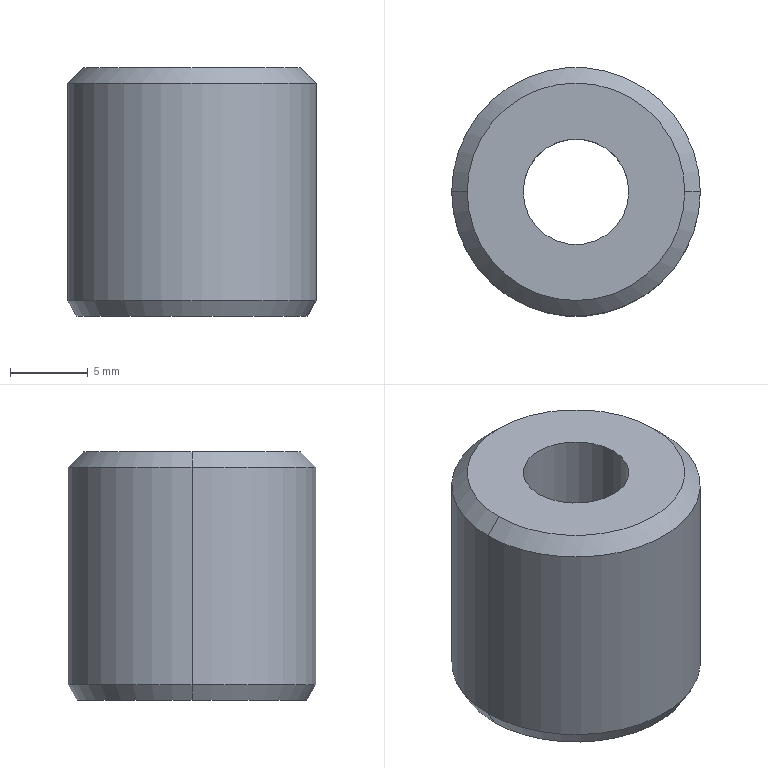Part | NX | features DCBA16_1 2 | 1 solid | 13 faces | box 16 x 16 x 16 mm | volume 2062 mm3 | cone 6 | cylinder 4 | plane 3 | commonest cylinder face diameters 16 x2 6.806 x1 11 x1
STEP:
#1=CARTESIAN_POINT('',(1522.268,-24.022,-21.001));
#2=VERTEX_POINT('',#1);
#3=CARTESIAN_POINT('',(1521.69,-24.022,-20.001));
#4=VERTEX_POINT('',#3);
#5=CARTESIAN_POINT('',(1521.69,-24.022,-20.001));
#6=DIRECTION('',(-0.5,0.,0.866));
#7=VECTOR('',#6,1000.);
#8=LINE('',#5,#7);
#9=EDGE_CURVE('',#2,#4,#8,.T.);
#10=ORIENTED_EDGE('',*,*,#9,.F.);
#11=CARTESIAN_POINT('',(1507.422,-24.022,-21.001));
#12=VERTEX_POINT('',#11);
#13=CARTESIAN_POINT('',(1514.845,-24.022,-21.001));
#14=DIRECTION('',(0.,0.,1.));
#15=DIRECTION('',(0.,1.,0.));
#16=AXIS2_PLACEMENT_3D('',#13,#14,#15);
#17=CIRCLE('',#16,7.423);
#18=EDGE_CURVE('',#2,#12,#17,.F.);
#19=ORIENTED_EDGE('',*,*,#18,.T.);
#20=CARTESIAN_POINT('',(1508.,-24.022,-20.001));
#21=VERTEX_POINT('',#20);
#22=CARTESIAN_POINT('',(1508.,-24.022,-20.001));
#23=DIRECTION('',(0.5,0.,0.866));
#24=VECTOR('',#23,1000.);
#25=LINE('',#22,#24);
#26=EDGE_CURVE('',#21,#12,#25,.F.);
#27=ORIENTED_EDGE('',*,*,#26,.F.);
#28=CARTESIAN_POINT('',(1514.845,-24.022,-20.001));
#29=DIRECTION('',(0.,0.,1.));
#30=DIRECTION('',(0.,1.,0.));
#31=AXIS2_PLACEMENT_3D('',#28,#29,#30);
#32=CIRCLE('',#31,6.845);
#33=EDGE_CURVE('',#4,#21,#32,.F.);
#34=ORIENTED_EDGE('',*,*,#33,.F.);
#35=EDGE_LOOP('',(#10,#19,#27,#34));
#36=FACE_BOUND('',#35,.T.);
#37=CARTESIAN_POINT('',(1514.845,-24.022,-20.001));
#38=DIRECTION('',(0.,0.,-1.));
#39=DIRECTION('',(-1.,0.,0.));
#40=AXIS2_PLACEMENT_3D('',#37,#38,#39);
#41=CONICAL_SURFACE('',#40,6.845,0.5236);
#42=ADVANCED_FACE('',(#36),#41,.F.);
#43=CARTESIAN_POINT('',(1522.845,-24.022,-20.001));
#44=VERTEX_POINT('',#43);
#45=CARTESIAN_POINT('',(1522.845,-24.022,-20.001));
#46=DIRECTION('',(-0.5,0.,-0.866));
#47=VECTOR('',#46,1000.);
#48=LINE('',#45,#47);
#49=EDGE_CURVE('',#44,#2,#48,.T.);
#50=ORIENTED_EDGE('',*,*,#49,.F.);
#51=CARTESIAN_POINT('',(1506.845,-24.022,-20.001));
#52=VERTEX_POINT('',#51);
#53=CARTESIAN_POINT('',(1514.845,-24.022,-20.001));
#54=DIRECTION('',(0.,0.,1.));
#55=DIRECTION('',(0.,1.,0.));
#56=AXIS2_PLACEMENT_3D('',#53,#54,#55);
#57=CIRCLE('',#56,8.);
#58=EDGE_CURVE('',#44,#52,#57,.F.);
#59=ORIENTED_EDGE('',*,*,#58,.T.);
#60=CARTESIAN_POINT('',(1506.845,-24.022,-20.001));
#61=DIRECTION('',(0.5,0.,-0.866));
#62=VECTOR('',#61,1000.);
#63=LINE('',#60,#62);
#64=EDGE_CURVE('',#12,#52,#63,.F.);
#65=ORIENTED_EDGE('',*,*,#64,.F.);
#66=ORIENTED_EDGE('',*,*,#18,.F.);
#67=EDGE_LOOP('',(#50,#59,#65,#66));
#68=FACE_BOUND('',#67,.T.);
#69=CARTESIAN_POINT('',(1514.845,-24.022,-20.001));
#70=DIRECTION('',(0.,0.,1.));
#71=DIRECTION('',(0.,1.,0.));
#72=AXIS2_PLACEMENT_3D('',#69,#70,#71);
#73=CONICAL_SURFACE('',#72,8.,0.5236);
#74=ADVANCED_FACE('',(#68),#73,.T.);
#75=ORIENTED_EDGE('',*,*,#49,.T.);
#76=CARTESIAN_POINT('',(1514.845,-24.022,-21.001));
#77=DIRECTION('',(0.,0.,1.));
#78=DIRECTION('',(0.,-1.,0.));
#79=AXIS2_PLACEMENT_3D('',#76,#77,#78);
#80=CIRCLE('',#79,7.423);
#81=EDGE_CURVE('',#12,#2,#80,.F.);
#82=ORIENTED_EDGE('',*,*,#81,.F.);
#83=ORIENTED_EDGE('',*,*,#64,.T.);
#84=CARTESIAN_POINT('',(1514.845,-24.022,-20.001));
#85=DIRECTION('',(0.,0.,1.));
#86=DIRECTION('',(0.,-1.,0.));
#87=AXIS2_PLACEMENT_3D('',#84,#85,#86);
#88=CIRCLE('',#87,8.);
#89=EDGE_CURVE('',#52,#44,#88,.F.);
#90=ORIENTED_EDGE('',*,*,#89,.T.);
#91=EDGE_LOOP('',(#75,#82,#83,#90));
#92=FACE_BOUND('',#91,.T.);
#93=CARTESIAN_POINT('',(1514.845,-24.022,-20.001));
#94=DIRECTION('',(0.,0.,1.));
#95=DIRECTION('',(0.,-1.,0.));
#96=AXIS2_PLACEMENT_3D('',#93,#94,#95);
#97=CONICAL_SURFACE('',#96,8.,0.5236);
#98=ADVANCED_FACE('',(#92),#97,.T.);
#99=ORIENTED_EDGE('',*,*,#9,.T.);
#100=CARTESIAN_POINT('',(1514.845,-24.022,-20.001));
#101=DIRECTION('',(0.,0.,1.));
#102=DIRECTION('',(0.,-1.,0.));
#103=AXIS2_PLACEMENT_3D('',#100,#101,#102);
#104=CIRCLE('',#103,6.845);
#105=EDGE_CURVE('',#21,#4,#104,.F.);
#106=ORIENTED_EDGE('',*,*,#105,.F.);
#107=ORIENTED_EDGE('',*,*,#26,.T.);
#108=ORIENTED_EDGE('',*,*,#81,.T.);
#109=EDGE_LOOP('',(#99,#106,#107,#108));
#110=FACE_BOUND('',#109,.T.);
#111=CARTESIAN_POINT('',(1514.845,-24.022,-21.001));
#112=DIRECTION('',(0.,0.,-1.));
#113=DIRECTION('',(0.,-1.,0.));
#114=AXIS2_PLACEMENT_3D('',#111,#112,#113);
#115=CONICAL_SURFACE('',#114,7.423,0.5236);
#116=ADVANCED_FACE('',(#110),#115,.F.);
#117=ORIENTED_EDGE('',*,*,#105,.T.);
#118=ORIENTED_EDGE('',*,*,#33,.T.);
#119=EDGE_LOOP('',(#117,#118));
#120=FACE_BOUND('',#119,.T.);
#121=CARTESIAN_POINT('',(1514.845,-18.522,-20.001));
#122=VERTEX_POINT('',#121);
#123=CARTESIAN_POINT('',(1514.845,-24.022,-20.001));
#124=DIRECTION('',(0.,0.,1.));
#125=DIRECTION('',(0.,1.,0.));
#126=AXIS2_PLACEMENT_3D('',#123,#124,#125);
#127=CIRCLE('',#126,5.5);
#128=EDGE_CURVE('',#122,#122,#127,.F.);
#129=ORIENTED_EDGE('',*,*,#128,.F.);
#130=EDGE_LOOP('',(#129));
#131=FACE_BOUND('',#130,.T.);
#132=CARTESIAN_POINT('',(1514.845,-24.022,-20.001));
#133=DIRECTION('',(0.,0.,-1.));
#134=DIRECTION('',(1.,0.,0.));
#135=AXIS2_PLACEMENT_3D('',#132,#133,#134);
#136=PLANE('',#135);
#137=ADVANCED_FACE('',(#120,#131),#136,.T.);
#138=ORIENTED_EDGE('',*,*,#128,.T.);
#139=EDGE_LOOP('',(#138));
#140=FACE_BOUND('',#139,.T.);
#141=CARTESIAN_POINT('',(1514.845,-29.522,-13.001));
#142=VERTEX_POINT('',#141);
#143=CARTESIAN_POINT('',(1514.845,-24.022,-13.001));
#144=DIRECTION('',(0.,0.,1.));
#145=DIRECTION('',(0.,-1.,0.));
#146=AXIS2_PLACEMENT_3D('',#143,#144,#145);
#147=CIRCLE('',#146,5.5);
#148=EDGE_CURVE('',#142,#142,#147,.F.);
#149=ORIENTED_EDGE('',*,*,#148,.F.);
#150=EDGE_LOOP('',(#149));
#151=FACE_BOUND('',#150,.T.);
#152=CARTESIAN_POINT('',(1514.845,-24.022,-20.001));
#153=DIRECTION('',(0.,0.,-1.));
#154=DIRECTION('',(0.,-1.,0.));
#155=AXIS2_PLACEMENT_3D('',#152,#153,#154);
#156=CYLINDRICAL_SURFACE('',#155,5.5);
#157=ADVANCED_FACE('',(#140,#151),#156,.F.);
#158=ORIENTED_EDGE('',*,*,#148,.T.);
#159=EDGE_LOOP('',(#158));
#160=FACE_BOUND('',#159,.T.);
#161=CARTESIAN_POINT('',(1511.442,-24.022,-13.001));
#162=VERTEX_POINT('',#161);
#163=CARTESIAN_POINT('',(1514.845,-24.022,-13.001));
#164=DIRECTION('',(0.,0.,1.));
#165=DIRECTION('',(-1.,0.,0.));
#166=AXIS2_PLACEMENT_3D('',#163,#164,#165);
#167=CIRCLE('',#166,3.403);
#168=EDGE_CURVE('',#162,#162,#167,.F.);
#169=ORIENTED_EDGE('',*,*,#168,.F.);
#170=EDGE_LOOP('',(#169));
#171=FACE_BOUND('',#170,.T.);
#172=CARTESIAN_POINT('',(1514.845,-24.022,-13.001));
#173=DIRECTION('',(0.,0.,-1.));
#174=DIRECTION('',(1.,0.,0.));
#175=AXIS2_PLACEMENT_3D('',#172,#173,#174);
#176=PLANE('',#175);
#177=ADVANCED_FACE('',(#160,#171),#176,.T.);
#178=ORIENTED_EDGE('',*,*,#168,.T.);
#179=EDGE_LOOP('',(#178));
#180=FACE_BOUND('',#179,.T.);
#181=CARTESIAN_POINT('',(1518.248,-24.022,-5.001));
#182=VERTEX_POINT('',#181);
#183=CARTESIAN_POINT('',(1514.845,-24.022,-5.001));
#184=DIRECTION('',(0.,0.,-1.));
#185=DIRECTION('',(1.,0.,0.));
#186=AXIS2_PLACEMENT_3D('',#183,#184,#185);
#187=CIRCLE('',#186,3.403);
#188=EDGE_CURVE('',#182,#182,#187,.T.);
#189=ORIENTED_EDGE('',*,*,#188,.F.);
#190=EDGE_LOOP('',(#189));
#191=FACE_BOUND('',#190,.T.);
#192=CARTESIAN_POINT('',(1514.845,-24.022,-13.001));
#193=DIRECTION('',(0.,0.,-1.));
#194=DIRECTION('',(0.,-1.,0.));
#195=AXIS2_PLACEMENT_3D('',#192,#193,#194);
#196=CYLINDRICAL_SURFACE('',#195,3.403);
#197=ADVANCED_FACE('',(#180,#191),#196,.F.);
#198=CARTESIAN_POINT('',(1521.845,-24.022,-5.001));
#199=VERTEX_POINT('',#198);
#200=CARTESIAN_POINT('',(1507.845,-24.022,-5.001));
#201=VERTEX_POINT('',#200);
#202=CARTESIAN_POINT('',(1514.845,-24.022,-5.001));
#203=DIRECTION('',(0.,0.,1.));
#204=DIRECTION('',(0.,1.,0.));
#205=AXIS2_PLACEMENT_3D('',#202,#203,#204);
#206=CIRCLE('',#205,7.);
#207=EDGE_CURVE('',#199,#201,#206,.F.);
#208=ORIENTED_EDGE('',*,*,#207,.F.);
#209=CARTESIAN_POINT('',(1514.845,-24.022,-5.001));
#210=DIRECTION('',(0.,0.,1.));
#211=DIRECTION('',(0.,-1.,0.));
#212=AXIS2_PLACEMENT_3D('',#209,#210,#211);
#213=CIRCLE('',#212,7.);
#214=EDGE_CURVE('',#201,#199,#213,.F.);
#215=ORIENTED_EDGE('',*,*,#214,.F.);
#216=EDGE_LOOP('',(#208,#215));
#217=FACE_BOUND('',#216,.T.);
#218=ORIENTED_EDGE('',*,*,#188,.T.);
#219=EDGE_LOOP('',(#218));
#220=FACE_BOUND('',#219,.T.);
#221=CARTESIAN_POINT('',(1514.845,-24.022,-5.001));
#222=DIRECTION('',(0.,0.,1.));
#223=DIRECTION('',(0.,-1.,0.));
#224=AXIS2_PLACEMENT_3D('',#221,#222,#223);
#225=PLANE('',#224);
#226=ADVANCED_FACE('',(#217,#220),#225,.T.);
#227=CARTESIAN_POINT('',(1522.845,-24.022,-6.001));
#228=VERTEX_POINT('',#227);
#229=CARTESIAN_POINT('',(1522.845,-24.022,-6.001));
#230=DIRECTION('',(0.7071,0.,-0.7071));
#231=VECTOR('',#230,1000.);
#232=LINE('',#229,#231);
#233=EDGE_CURVE('',#199,#228,#232,.T.);
#234=ORIENTED_EDGE('',*,*,#233,.F.);
#235=ORIENTED_EDGE('',*,*,#207,.T.);
#236=CARTESIAN_POINT('',(1506.845,-24.022,-6.001));
#237=VERTEX_POINT('',#236);
#238=CARTESIAN_POINT('',(1506.845,-24.022,-6.001));
#239=DIRECTION('',(-0.7071,0.,-0.7071));
#240=VECTOR('',#239,1000.);
#241=LINE('',#238,#240);
#242=EDGE_CURVE('',#237,#201,#241,.F.);
#243=ORIENTED_EDGE('',*,*,#242,.F.);
#244=CARTESIAN_POINT('',(1514.845,-24.022,-6.001));
#245=DIRECTION('',(0.,0.,1.));
#246=DIRECTION('',(0.,1.,0.));
#247=AXIS2_PLACEMENT_3D('',#244,#245,#246);
#248=CIRCLE('',#247,8.);
#249=EDGE_CURVE('',#228,#237,#248,.F.);
#250=ORIENTED_EDGE('',*,*,#249,.F.);
#251=EDGE_LOOP('',(#234,#235,#243,#250));
#252=FACE_BOUND('',#251,.T.);
#253=CARTESIAN_POINT('',(1514.845,-24.022,-6.001));
#254=DIRECTION('',(0.,0.,-1.));
#255=DIRECTION('',(0.,1.,0.));
#256=AXIS2_PLACEMENT_3D('',#253,#254,#255);
#257=CONICAL_SURFACE('',#256,8.,0.7854);
#258=ADVANCED_FACE('',(#252),#257,.T.);
#259=ORIENTED_EDGE('',*,*,#233,.T.);
#260=CARTESIAN_POINT('',(1514.845,-24.022,-6.001));
#261=DIRECTION('',(0.,0.,1.));
#262=DIRECTION('',(0.,-1.,0.));
#263=AXIS2_PLACEMENT_3D('',#260,#261,#262);
#264=CIRCLE('',#263,8.);
#265=EDGE_CURVE('',#237,#228,#264,.F.);
#266=ORIENTED_EDGE('',*,*,#265,.F.);
#267=ORIENTED_EDGE('',*,*,#242,.T.);
#268=ORIENTED_EDGE('',*,*,#214,.T.);
#269=EDGE_LOOP('',(#259,#266,#267,#268));
#270=FACE_BOUND('',#269,.T.);
#271=CARTESIAN_POINT('',(1514.845,-24.022,-6.001));
#272=DIRECTION('',(0.,0.,-1.));
#273=DIRECTION('',(0.,-1.,0.));
#274=AXIS2_PLACEMENT_3D('',#271,#272,#273);
#275=CONICAL_SURFACE('',#274,8.,0.7854);
#276=ADVANCED_FACE('',(#270),#275,.T.);
#277=CARTESIAN_POINT('',(1522.845,-24.022,-6.001));
#278=DIRECTION('',(0.,0.,-1.));
#279=VECTOR('',#278,1000.);
#280=LINE('',#277,#279);
#281=EDGE_CURVE('',#44,#228,#280,.F.);
#282=ORIENTED_EDGE('',*,*,#281,.T.);
#283=ORIENTED_EDGE('',*,*,#249,.T.);
#284=CARTESIAN_POINT('',(1506.845,-24.022,-6.001));
#285=DIRECTION('',(0.,0.,-1.));
#286=VECTOR('',#285,1000.);
#287=LINE('',#284,#286);
#288=EDGE_CURVE('',#237,#52,#287,.T.);
#289=ORIENTED_EDGE('',*,*,#288,.T.);
#290=ORIENTED_EDGE('',*,*,#58,.F.);
#291=EDGE_LOOP('',(#282,#283,#289,#290));
#292=FACE_BOUND('',#291,.T.);
#293=CARTESIAN_POINT('',(1514.845,-24.022,-6.001));
#294=DIRECTION('',(0.,0.,1.));
#295=DIRECTION('',(0.,1.,0.));
#296=AXIS2_PLACEMENT_3D('',#293,#294,#295);
#297=CYLINDRICAL_SURFACE('',#296,8.);
#298=ADVANCED_FACE('',(#292),#297,.T.);
#299=ORIENTED_EDGE('',*,*,#281,.F.);
#300=ORIENTED_EDGE('',*,*,#89,.F.);
#301=ORIENTED_EDGE('',*,*,#288,.F.);
#302=ORIENTED_EDGE('',*,*,#265,.T.);
#303=EDGE_LOOP('',(#299,#300,#301,#302));
#304=FACE_BOUND('',#303,.T.);
#305=CARTESIAN_POINT('',(1514.845,-24.022,-6.001));
#306=DIRECTION('',(0.,0.,1.));
#307=DIRECTION('',(0.,-1.,0.));
#308=AXIS2_PLACEMENT_3D('',#305,#306,#307);
#309=CYLINDRICAL_SURFACE('',#308,8.);
#310=ADVANCED_FACE('',(#304),#309,.T.);
#311=CLOSED_SHELL('',(#42,#74,#98,#116,#137,#157,#177,#197,#226,#258,#276,#298,#310));
#312=MANIFOLD_SOLID_BREP('',#311);
#313=(LENGTH_UNIT()NAMED_UNIT(*)SI_UNIT(.MILLI.,.METRE.));
#314=UNCERTAINTY_MEASURE_WITH_UNIT(LENGTH_MEASURE(0.00001),#313,'','');
#315=(NAMED_UNIT(*)PLANE_ANGLE_UNIT()SI_UNIT($,.RADIAN.));
#316=(NAMED_UNIT(*)SI_UNIT($,.STERADIAN.)SOLID_ANGLE_UNIT());
#317=(GEOMETRIC_REPRESENTATION_CONTEXT(3)GLOBAL_UNCERTAINTY_ASSIGNED_CONTEXT((#314))GLOBAL_UNIT_ASSIGNED_CONTEXT((#313,#315,#316))REPRESENTATION_CONTEXT('',''));
#318=ADVANCED_BREP_SHAPE_REPRESENTATION('',(#312),#317);